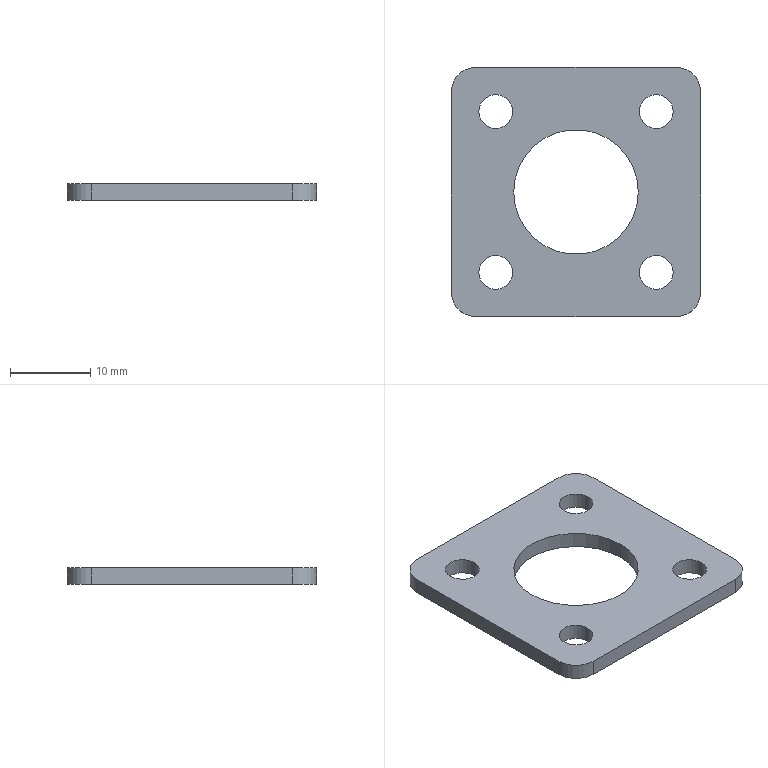Part | NX | features BREP 1 | 1 solid | 20 faces | box 31 x 31 x 2 mm | volume 1418 mm3 | cylinder 14 | plane 6 | commonest cylinder face diameters 4.2 x8 6 x4 15.5 x2
STEP:
#1=CARTESIAN_POINT('',(-258.211,-178.403,2108.));
#2=VERTEX_POINT('',#1);
#3=CARTESIAN_POINT('',(-262.411,-178.403,2108.));
#4=VERTEX_POINT('',#3);
#5=CARTESIAN_POINT('',(-260.311,-178.403,2108.));
#6=DIRECTION('',(0.,0.,-1.));
#7=DIRECTION('',(-1.,0.,0.));
#8=AXIS2_PLACEMENT_3D('',#5,#6,#7);
#9=CIRCLE('',#8,2.1);
#10=EDGE_CURVE('',#2,#4,#9,.T.);
#11=ORIENTED_EDGE('',*,*,#10,.F.);
#12=CARTESIAN_POINT('',(-258.211,-178.403,2106.));
#13=VERTEX_POINT('',#12);
#14=CARTESIAN_POINT('',(-258.211,-178.403,2108.));
#15=DIRECTION('',(0.,0.,-1.));
#16=VECTOR('',#15,1000.);
#17=LINE('',#14,#16);
#18=EDGE_CURVE('',#13,#2,#17,.F.);
#19=ORIENTED_EDGE('',*,*,#18,.F.);
#20=CARTESIAN_POINT('',(-262.411,-178.403,2106.));
#21=VERTEX_POINT('',#20);
#22=CARTESIAN_POINT('',(-260.311,-178.403,2106.));
#23=DIRECTION('',(0.,0.,1.));
#24=DIRECTION('',(-1.,0.,0.));
#25=AXIS2_PLACEMENT_3D('',#22,#23,#24);
#26=CIRCLE('',#25,2.1);
#27=EDGE_CURVE('',#21,#13,#26,.T.);
#28=ORIENTED_EDGE('',*,*,#27,.F.);
#29=CARTESIAN_POINT('',(-262.411,-178.403,2108.));
#30=DIRECTION('',(0.,0.,-1.));
#31=VECTOR('',#30,1000.);
#32=LINE('',#29,#31);
#33=EDGE_CURVE('',#21,#4,#32,.F.);
#34=ORIENTED_EDGE('',*,*,#33,.T.);
#35=EDGE_LOOP('',(#11,#19,#28,#34));
#36=FACE_BOUND('',#35,.T.);
#37=CARTESIAN_POINT('',(-260.311,-178.403,2108.));
#38=DIRECTION('',(0.,0.,-1.));
#39=DIRECTION('',(1.,0.,0.));
#40=AXIS2_PLACEMENT_3D('',#37,#38,#39);
#41=CYLINDRICAL_SURFACE('',#40,2.1);
#42=ADVANCED_FACE('',(#36),#41,.F.);
#43=CARTESIAN_POINT('',(-238.211,-198.403,2108.));
#44=VERTEX_POINT('',#43);
#45=CARTESIAN_POINT('',(-242.411,-198.403,2108.));
#46=VERTEX_POINT('',#45);
#47=CARTESIAN_POINT('',(-240.311,-198.403,2108.));
#48=DIRECTION('',(0.,0.,-1.));
#49=DIRECTION('',(-1.,0.,0.));
#50=AXIS2_PLACEMENT_3D('',#47,#48,#49);
#51=CIRCLE('',#50,2.1);
#52=EDGE_CURVE('',#44,#46,#51,.T.);
#53=ORIENTED_EDGE('',*,*,#52,.F.);
#54=CARTESIAN_POINT('',(-238.211,-198.403,2106.));
#55=VERTEX_POINT('',#54);
#56=CARTESIAN_POINT('',(-238.211,-198.403,2108.));
#57=DIRECTION('',(0.,0.,-1.));
#58=VECTOR('',#57,1000.);
#59=LINE('',#56,#58);
#60=EDGE_CURVE('',#55,#44,#59,.F.);
#61=ORIENTED_EDGE('',*,*,#60,.F.);
#62=CARTESIAN_POINT('',(-242.411,-198.403,2106.));
#63=VERTEX_POINT('',#62);
#64=CARTESIAN_POINT('',(-240.311,-198.403,2106.));
#65=DIRECTION('',(0.,0.,1.));
#66=DIRECTION('',(-1.,0.,0.));
#67=AXIS2_PLACEMENT_3D('',#64,#65,#66);
#68=CIRCLE('',#67,2.1);
#69=EDGE_CURVE('',#63,#55,#68,.T.);
#70=ORIENTED_EDGE('',*,*,#69,.F.);
#71=CARTESIAN_POINT('',(-242.411,-198.403,2108.));
#72=DIRECTION('',(0.,0.,-1.));
#73=VECTOR('',#72,1000.);
#74=LINE('',#71,#73);
#75=EDGE_CURVE('',#63,#46,#74,.F.);
#76=ORIENTED_EDGE('',*,*,#75,.T.);
#77=EDGE_LOOP('',(#53,#61,#70,#76));
#78=FACE_BOUND('',#77,.T.);
#79=CARTESIAN_POINT('',(-240.311,-198.403,2108.));
#80=DIRECTION('',(0.,0.,-1.));
#81=DIRECTION('',(1.,0.,0.));
#82=AXIS2_PLACEMENT_3D('',#79,#80,#81);
#83=CYLINDRICAL_SURFACE('',#82,2.1);
#84=ADVANCED_FACE('',(#78),#83,.F.);
#85=CARTESIAN_POINT('',(-242.561,-188.403,2108.));
#86=VERTEX_POINT('',#85);
#87=CARTESIAN_POINT('',(-258.061,-188.403,2108.));
#88=VERTEX_POINT('',#87);
#89=CARTESIAN_POINT('',(-250.311,-188.403,2108.));
#90=DIRECTION('',(0.,0.,-1.));
#91=DIRECTION('',(-1.,0.,0.));
#92=AXIS2_PLACEMENT_3D('',#89,#90,#91);
#93=CIRCLE('',#92,7.75);
#94=EDGE_CURVE('',#86,#88,#93,.T.);
#95=ORIENTED_EDGE('',*,*,#94,.F.);
#96=CARTESIAN_POINT('',(-242.561,-188.403,2106.));
#97=VERTEX_POINT('',#96);
#98=CARTESIAN_POINT('',(-242.561,-188.403,2108.));
#99=DIRECTION('',(0.,0.,-1.));
#100=VECTOR('',#99,1000.);
#101=LINE('',#98,#100);
#102=EDGE_CURVE('',#97,#86,#101,.F.);
#103=ORIENTED_EDGE('',*,*,#102,.F.);
#104=CARTESIAN_POINT('',(-258.061,-188.403,2106.));
#105=VERTEX_POINT('',#104);
#106=CARTESIAN_POINT('',(-250.311,-188.403,2106.));
#107=DIRECTION('',(0.,0.,1.));
#108=DIRECTION('',(-1.,0.,0.));
#109=AXIS2_PLACEMENT_3D('',#106,#107,#108);
#110=CIRCLE('',#109,7.75);
#111=EDGE_CURVE('',#105,#97,#110,.T.);
#112=ORIENTED_EDGE('',*,*,#111,.F.);
#113=CARTESIAN_POINT('',(-258.061,-188.403,2108.));
#114=DIRECTION('',(0.,0.,-1.));
#115=VECTOR('',#114,1000.);
#116=LINE('',#113,#115);
#117=EDGE_CURVE('',#105,#88,#116,.F.);
#118=ORIENTED_EDGE('',*,*,#117,.T.);
#119=EDGE_LOOP('',(#95,#103,#112,#118));
#120=FACE_BOUND('',#119,.T.);
#121=CARTESIAN_POINT('',(-250.311,-188.403,2108.));
#122=DIRECTION('',(0.,0.,-1.));
#123=DIRECTION('',(1.,0.,0.));
#124=AXIS2_PLACEMENT_3D('',#121,#122,#123);
#125=CYLINDRICAL_SURFACE('',#124,7.75);
#126=ADVANCED_FACE('',(#120),#125,.F.);
#127=CARTESIAN_POINT('',(-238.211,-178.403,2108.));
#128=VERTEX_POINT('',#127);
#129=CARTESIAN_POINT('',(-242.411,-178.403,2108.));
#130=VERTEX_POINT('',#129);
#131=CARTESIAN_POINT('',(-240.311,-178.403,2108.));
#132=DIRECTION('',(0.,0.,-1.));
#133=DIRECTION('',(-1.,0.,0.));
#134=AXIS2_PLACEMENT_3D('',#131,#132,#133);
#135=CIRCLE('',#134,2.1);
#136=EDGE_CURVE('',#128,#130,#135,.T.);
#137=ORIENTED_EDGE('',*,*,#136,.F.);
#138=CARTESIAN_POINT('',(-238.211,-178.403,2106.));
#139=VERTEX_POINT('',#138);
#140=CARTESIAN_POINT('',(-238.211,-178.403,2108.));
#141=DIRECTION('',(0.,0.,-1.));
#142=VECTOR('',#141,1000.);
#143=LINE('',#140,#142);
#144=EDGE_CURVE('',#139,#128,#143,.F.);
#145=ORIENTED_EDGE('',*,*,#144,.F.);
#146=CARTESIAN_POINT('',(-242.411,-178.403,2106.));
#147=VERTEX_POINT('',#146);
#148=CARTESIAN_POINT('',(-240.311,-178.403,2106.));
#149=DIRECTION('',(0.,0.,1.));
#150=DIRECTION('',(-1.,0.,0.));
#151=AXIS2_PLACEMENT_3D('',#148,#149,#150);
#152=CIRCLE('',#151,2.1);
#153=EDGE_CURVE('',#147,#139,#152,.T.);
#154=ORIENTED_EDGE('',*,*,#153,.F.);
#155=CARTESIAN_POINT('',(-242.411,-178.403,2108.));
#156=DIRECTION('',(0.,0.,-1.));
#157=VECTOR('',#156,1000.);
#158=LINE('',#155,#157);
#159=EDGE_CURVE('',#147,#130,#158,.F.);
#160=ORIENTED_EDGE('',*,*,#159,.T.);
#161=EDGE_LOOP('',(#137,#145,#154,#160));
#162=FACE_BOUND('',#161,.T.);
#163=CARTESIAN_POINT('',(-240.311,-178.403,2108.));
#164=DIRECTION('',(0.,0.,-1.));
#165=DIRECTION('',(1.,0.,0.));
#166=AXIS2_PLACEMENT_3D('',#163,#164,#165);
#167=CYLINDRICAL_SURFACE('',#166,2.1);
#168=ADVANCED_FACE('',(#162),#167,.F.);
#169=CARTESIAN_POINT('',(-258.211,-198.403,2108.));
#170=VERTEX_POINT('',#169);
#171=CARTESIAN_POINT('',(-262.411,-198.403,2108.));
#172=VERTEX_POINT('',#171);
#173=CARTESIAN_POINT('',(-260.311,-198.403,2108.));
#174=DIRECTION('',(0.,0.,-1.));
#175=DIRECTION('',(-1.,0.,0.));
#176=AXIS2_PLACEMENT_3D('',#173,#174,#175);
#177=CIRCLE('',#176,2.1);
#178=EDGE_CURVE('',#170,#172,#177,.T.);
#179=ORIENTED_EDGE('',*,*,#178,.F.);
#180=CARTESIAN_POINT('',(-258.211,-198.403,2106.));
#181=VERTEX_POINT('',#180);
#182=CARTESIAN_POINT('',(-258.211,-198.403,2108.));
#183=DIRECTION('',(0.,0.,-1.));
#184=VECTOR('',#183,1000.);
#185=LINE('',#182,#184);
#186=EDGE_CURVE('',#181,#170,#185,.F.);
#187=ORIENTED_EDGE('',*,*,#186,.F.);
#188=CARTESIAN_POINT('',(-262.411,-198.403,2106.));
#189=VERTEX_POINT('',#188);
#190=CARTESIAN_POINT('',(-260.311,-198.403,2106.));
#191=DIRECTION('',(0.,0.,1.));
#192=DIRECTION('',(-1.,0.,0.));
#193=AXIS2_PLACEMENT_3D('',#190,#191,#192);
#194=CIRCLE('',#193,2.1);
#195=EDGE_CURVE('',#189,#181,#194,.T.);
#196=ORIENTED_EDGE('',*,*,#195,.F.);
#197=CARTESIAN_POINT('',(-262.411,-198.403,2108.));
#198=DIRECTION('',(0.,0.,-1.));
#199=VECTOR('',#198,1000.);
#200=LINE('',#197,#199);
#201=EDGE_CURVE('',#189,#172,#200,.F.);
#202=ORIENTED_EDGE('',*,*,#201,.T.);
#203=EDGE_LOOP('',(#179,#187,#196,#202));
#204=FACE_BOUND('',#203,.T.);
#205=CARTESIAN_POINT('',(-260.311,-198.403,2108.));
#206=DIRECTION('',(0.,0.,-1.));
#207=DIRECTION('',(1.,0.,0.));
#208=AXIS2_PLACEMENT_3D('',#205,#206,#207);
#209=CYLINDRICAL_SURFACE('',#208,2.1);
#210=ADVANCED_FACE('',(#204),#209,.F.);
#211=CARTESIAN_POINT('',(-234.811,-175.903,2108.));
#212=VERTEX_POINT('',#211);
#213=CARTESIAN_POINT('',(-237.811,-172.903,2108.));
#214=VERTEX_POINT('',#213);
#215=CARTESIAN_POINT('',(-237.811,-175.903,2108.));
#216=DIRECTION('',(0.,0.,1.));
#217=DIRECTION('',(1.,0.,0.));
#218=AXIS2_PLACEMENT_3D('',#215,#216,#217);
#219=CIRCLE('',#218,3.);
#220=EDGE_CURVE('',#212,#214,#219,.T.);
#221=ORIENTED_EDGE('',*,*,#220,.T.);
#222=CARTESIAN_POINT('',(-262.811,-172.903,2108.));
#223=VERTEX_POINT('',#222);
#224=CARTESIAN_POINT('',(-237.311,-172.903,2108.));
#225=DIRECTION('',(-1.,0.,0.));
#226=VECTOR('',#225,1000.);
#227=LINE('',#224,#226);
#228=EDGE_CURVE('',#214,#223,#227,.T.);
#229=ORIENTED_EDGE('',*,*,#228,.T.);
#230=CARTESIAN_POINT('',(-265.811,-175.903,2108.));
#231=VERTEX_POINT('',#230);
#232=CARTESIAN_POINT('',(-262.811,-175.903,2108.));
#233=DIRECTION('',(0.,0.,1.));
#234=DIRECTION('',(1.,0.,0.));
#235=AXIS2_PLACEMENT_3D('',#232,#233,#234);
#236=CIRCLE('',#235,3.);
#237=EDGE_CURVE('',#223,#231,#236,.T.);
#238=ORIENTED_EDGE('',*,*,#237,.T.);
#239=CARTESIAN_POINT('',(-265.811,-200.903,2108.));
#240=VERTEX_POINT('',#239);
#241=CARTESIAN_POINT('',(-265.811,-201.403,2108.));
#242=DIRECTION('',(0.,-1.,0.));
#243=VECTOR('',#242,1000.);
#244=LINE('',#241,#243);
#245=EDGE_CURVE('',#231,#240,#244,.T.);
#246=ORIENTED_EDGE('',*,*,#245,.T.);
#247=CARTESIAN_POINT('',(-262.811,-203.903,2108.));
#248=VERTEX_POINT('',#247);
#249=CARTESIAN_POINT('',(-262.811,-200.903,2108.));
#250=DIRECTION('',(0.,0.,1.));
#251=DIRECTION('',(1.,0.,0.));
#252=AXIS2_PLACEMENT_3D('',#249,#250,#251);
#253=CIRCLE('',#252,3.);
#254=EDGE_CURVE('',#240,#248,#253,.T.);
#255=ORIENTED_EDGE('',*,*,#254,.T.);
#256=CARTESIAN_POINT('',(-237.811,-203.903,2108.));
#257=VERTEX_POINT('',#256);
#258=CARTESIAN_POINT('',(-237.311,-203.903,2108.));
#259=DIRECTION('',(1.,0.,0.));
#260=VECTOR('',#259,1000.);
#261=LINE('',#258,#260);
#262=EDGE_CURVE('',#248,#257,#261,.T.);
#263=ORIENTED_EDGE('',*,*,#262,.T.);
#264=CARTESIAN_POINT('',(-234.811,-200.903,2108.));
#265=VERTEX_POINT('',#264);
#266=CARTESIAN_POINT('',(-237.811,-200.903,2108.));
#267=DIRECTION('',(0.,0.,1.));
#268=DIRECTION('',(1.,0.,0.));
#269=AXIS2_PLACEMENT_3D('',#266,#267,#268);
#270=CIRCLE('',#269,3.);
#271=EDGE_CURVE('',#257,#265,#270,.T.);
#272=ORIENTED_EDGE('',*,*,#271,.T.);
#273=CARTESIAN_POINT('',(-234.811,-201.403,2108.));
#274=DIRECTION('',(0.,1.,0.));
#275=VECTOR('',#274,1000.);
#276=LINE('',#273,#275);
#277=EDGE_CURVE('',#265,#212,#276,.T.);
#278=ORIENTED_EDGE('',*,*,#277,.T.);
#279=EDGE_LOOP('',(#221,#229,#238,#246,#255,#263,#272,#278));
#280=FACE_BOUND('',#279,.T.);
#281=CARTESIAN_POINT('',(-260.311,-178.403,2108.));
#282=DIRECTION('',(0.,0.,-1.));
#283=DIRECTION('',(-1.,0.,0.));
#284=AXIS2_PLACEMENT_3D('',#281,#282,#283);
#285=CIRCLE('',#284,2.1);
#286=EDGE_CURVE('',#4,#2,#285,.T.);
#287=ORIENTED_EDGE('',*,*,#286,.T.);
#288=ORIENTED_EDGE('',*,*,#10,.T.);
#289=EDGE_LOOP('',(#287,#288));
#290=FACE_BOUND('',#289,.T.);
#291=CARTESIAN_POINT('',(-240.311,-198.403,2108.));
#292=DIRECTION('',(0.,0.,-1.));
#293=DIRECTION('',(-1.,0.,0.));
#294=AXIS2_PLACEMENT_3D('',#291,#292,#293);
#295=CIRCLE('',#294,2.1);
#296=EDGE_CURVE('',#46,#44,#295,.T.);
#297=ORIENTED_EDGE('',*,*,#296,.T.);
#298=ORIENTED_EDGE('',*,*,#52,.T.);
#299=EDGE_LOOP('',(#297,#298));
#300=FACE_BOUND('',#299,.T.);
#301=CARTESIAN_POINT('',(-250.311,-188.403,2108.));
#302=DIRECTION('',(0.,0.,-1.));
#303=DIRECTION('',(-1.,0.,0.));
#304=AXIS2_PLACEMENT_3D('',#301,#302,#303);
#305=CIRCLE('',#304,7.75);
#306=EDGE_CURVE('',#88,#86,#305,.T.);
#307=ORIENTED_EDGE('',*,*,#306,.T.);
#308=ORIENTED_EDGE('',*,*,#94,.T.);
#309=EDGE_LOOP('',(#307,#308));
#310=FACE_BOUND('',#309,.T.);
#311=CARTESIAN_POINT('',(-240.311,-178.403,2108.));
#312=DIRECTION('',(0.,0.,-1.));
#313=DIRECTION('',(-1.,0.,0.));
#314=AXIS2_PLACEMENT_3D('',#311,#312,#313);
#315=CIRCLE('',#314,2.1);
#316=EDGE_CURVE('',#130,#128,#315,.T.);
#317=ORIENTED_EDGE('',*,*,#316,.T.);
#318=ORIENTED_EDGE('',*,*,#136,.T.);
#319=EDGE_LOOP('',(#317,#318));
#320=FACE_BOUND('',#319,.T.);
#321=CARTESIAN_POINT('',(-260.311,-198.403,2108.));
#322=DIRECTION('',(0.,0.,-1.));
#323=DIRECTION('',(-1.,0.,0.));
#324=AXIS2_PLACEMENT_3D('',#321,#322,#323);
#325=CIRCLE('',#324,2.1);
#326=EDGE_CURVE('',#172,#170,#325,.T.);
#327=ORIENTED_EDGE('',*,*,#326,.T.);
#328=ORIENTED_EDGE('',*,*,#178,.T.);
#329=EDGE_LOOP('',(#327,#328));
#330=FACE_BOUND('',#329,.T.);
#331=CARTESIAN_POINT('',(-237.311,-201.403,2108.));
#332=DIRECTION('',(0.,0.,1.));
#333=DIRECTION('',(-1.,0.,0.));
#334=AXIS2_PLACEMENT_3D('',#331,#332,#333);
#335=PLANE('',#334);
#336=ADVANCED_FACE('',(#280,#290,#300,#310,#320,#330),#335,.T.);
#337=CARTESIAN_POINT('',(-237.811,-172.903,2106.));
#338=VERTEX_POINT('',#337);
#339=CARTESIAN_POINT('',(-237.811,-172.903,2098.));
#340=DIRECTION('',(0.,0.,1.));
#341=VECTOR('',#340,1000.);
#342=LINE('',#339,#341);
#343=EDGE_CURVE('',#338,#214,#342,.T.);
#344=ORIENTED_EDGE('',*,*,#343,.F.);
#345=CARTESIAN_POINT('',(-262.811,-172.903,2106.));
#346=VERTEX_POINT('',#345);
#347=CARTESIAN_POINT('',(-250.311,-172.903,2106.));
#348=DIRECTION('',(1.,0.,0.));
#349=VECTOR('',#348,1000.);
#350=LINE('',#347,#349);
#351=EDGE_CURVE('',#346,#338,#350,.T.);
#352=ORIENTED_EDGE('',*,*,#351,.F.);
#353=CARTESIAN_POINT('',(-262.811,-172.903,2098.));
#354=DIRECTION('',(0.,0.,-1.));
#355=VECTOR('',#354,1000.);
#356=LINE('',#353,#355);
#357=EDGE_CURVE('',#223,#346,#356,.T.);
#358=ORIENTED_EDGE('',*,*,#357,.F.);
#359=ORIENTED_EDGE('',*,*,#228,.F.);
#360=EDGE_LOOP('',(#344,#352,#358,#359));
#361=FACE_BOUND('',#360,.T.);
#362=CARTESIAN_POINT('',(-250.311,-172.903,2098.));
#363=DIRECTION('',(0.,-1.,0.));
#364=DIRECTION('',(0.,0.,1.));
#365=AXIS2_PLACEMENT_3D('',#362,#363,#364);
#366=PLANE('',#365);
#367=ADVANCED_FACE('',(#361),#366,.F.);
#368=ORIENTED_EDGE('',*,*,#343,.T.);
#369=ORIENTED_EDGE('',*,*,#220,.F.);
#370=CARTESIAN_POINT('',(-234.811,-175.903,2106.));
#371=VERTEX_POINT('',#370);
#372=CARTESIAN_POINT('',(-234.811,-175.903,2098.));
#373=DIRECTION('',(0.,0.,-1.));
#374=VECTOR('',#373,1000.);
#375=LINE('',#372,#374);
#376=EDGE_CURVE('',#212,#371,#375,.T.);
#377=ORIENTED_EDGE('',*,*,#376,.T.);
#378=CARTESIAN_POINT('',(-237.811,-175.903,2106.));
#379=DIRECTION('',(0.,0.,1.));
#380=DIRECTION('',(1.,0.,0.));
#381=AXIS2_PLACEMENT_3D('',#378,#379,#380);
#382=CIRCLE('',#381,3.);
#383=EDGE_CURVE('',#371,#338,#382,.T.);
#384=ORIENTED_EDGE('',*,*,#383,.T.);
#385=EDGE_LOOP('',(#368,#369,#377,#384));
#386=FACE_BOUND('',#385,.T.);
#387=CARTESIAN_POINT('',(-237.811,-175.903,2098.));
#388=DIRECTION('',(0.,0.,1.));
#389=DIRECTION('',(-1.,0.,0.));
#390=AXIS2_PLACEMENT_3D('',#387,#388,#389);
#391=CYLINDRICAL_SURFACE('',#390,3.);
#392=ADVANCED_FACE('',(#386),#391,.T.);
#393=ORIENTED_EDGE('',*,*,#277,.F.);
#394=CARTESIAN_POINT('',(-234.811,-200.903,2106.));
#395=VERTEX_POINT('',#394);
#396=CARTESIAN_POINT('',(-234.811,-200.903,2098.));
#397=DIRECTION('',(0.,0.,-1.));
#398=VECTOR('',#397,1000.);
#399=LINE('',#396,#398);
#400=EDGE_CURVE('',#265,#395,#399,.T.);
#401=ORIENTED_EDGE('',*,*,#400,.T.);
#402=CARTESIAN_POINT('',(-234.811,-188.403,2106.));
#403=DIRECTION('',(0.,1.,0.));
#404=VECTOR('',#403,1000.);
#405=LINE('',#402,#404);
#406=EDGE_CURVE('',#395,#371,#405,.T.);
#407=ORIENTED_EDGE('',*,*,#406,.T.);
#408=ORIENTED_EDGE('',*,*,#376,.F.);
#409=EDGE_LOOP('',(#393,#401,#407,#408));
#410=FACE_BOUND('',#409,.T.);
#411=CARTESIAN_POINT('',(-234.811,-188.403,2098.));
#412=DIRECTION('',(1.,0.,0.));
#413=DIRECTION('',(0.,0.,1.));
#414=AXIS2_PLACEMENT_3D('',#411,#412,#413);
#415=PLANE('',#414);
#416=ADVANCED_FACE('',(#410),#415,.T.);
#417=ORIENTED_EDGE('',*,*,#400,.F.);
#418=ORIENTED_EDGE('',*,*,#271,.F.);
#419=CARTESIAN_POINT('',(-237.811,-203.903,2106.));
#420=VERTEX_POINT('',#419);
#421=CARTESIAN_POINT('',(-237.811,-203.903,2098.));
#422=DIRECTION('',(0.,0.,-1.));
#423=VECTOR('',#422,1000.);
#424=LINE('',#421,#423);
#425=EDGE_CURVE('',#257,#420,#424,.T.);
#426=ORIENTED_EDGE('',*,*,#425,.T.);
#427=CARTESIAN_POINT('',(-237.811,-200.903,2106.));
#428=DIRECTION('',(0.,0.,1.));
#429=DIRECTION('',(1.,0.,0.));
#430=AXIS2_PLACEMENT_3D('',#427,#428,#429);
#431=CIRCLE('',#430,3.);
#432=EDGE_CURVE('',#420,#395,#431,.T.);
#433=ORIENTED_EDGE('',*,*,#432,.T.);
#434=EDGE_LOOP('',(#417,#418,#426,#433));
#435=FACE_BOUND('',#434,.T.);
#436=CARTESIAN_POINT('',(-237.811,-200.903,2098.));
#437=DIRECTION('',(0.,0.,1.));
#438=DIRECTION('',(-1.,0.,0.));
#439=AXIS2_PLACEMENT_3D('',#436,#437,#438);
#440=CYLINDRICAL_SURFACE('',#439,3.);
#441=ADVANCED_FACE('',(#435),#440,.T.);
#442=ORIENTED_EDGE('',*,*,#262,.F.);
#443=CARTESIAN_POINT('',(-262.811,-203.903,2106.));
#444=VERTEX_POINT('',#443);
#445=CARTESIAN_POINT('',(-262.811,-203.903,2098.));
#446=DIRECTION('',(0.,0.,-1.));
#447=VECTOR('',#446,1000.);
#448=LINE('',#445,#447);
#449=EDGE_CURVE('',#248,#444,#448,.T.);
#450=ORIENTED_EDGE('',*,*,#449,.T.);
#451=CARTESIAN_POINT('',(-250.311,-203.903,2106.));
#452=DIRECTION('',(1.,0.,0.));
#453=VECTOR('',#452,1000.);
#454=LINE('',#451,#453);
#455=EDGE_CURVE('',#444,#420,#454,.T.);
#456=ORIENTED_EDGE('',*,*,#455,.T.);
#457=ORIENTED_EDGE('',*,*,#425,.F.);
#458=EDGE_LOOP('',(#442,#450,#456,#457));
#459=FACE_BOUND('',#458,.T.);
#460=CARTESIAN_POINT('',(-250.311,-203.903,2098.));
#461=DIRECTION('',(0.,-1.,0.));
#462=DIRECTION('',(0.,0.,1.));
#463=AXIS2_PLACEMENT_3D('',#460,#461,#462);
#464=PLANE('',#463);
#465=ADVANCED_FACE('',(#459),#464,.T.);
#466=ORIENTED_EDGE('',*,*,#449,.F.);
#467=ORIENTED_EDGE('',*,*,#254,.F.);
#468=CARTESIAN_POINT('',(-265.811,-200.903,2106.));
#469=VERTEX_POINT('',#468);
#470=CARTESIAN_POINT('',(-265.811,-200.903,2098.));
#471=DIRECTION('',(0.,0.,-1.));
#472=VECTOR('',#471,1000.);
#473=LINE('',#470,#472);
#474=EDGE_CURVE('',#240,#469,#473,.T.);
#475=ORIENTED_EDGE('',*,*,#474,.T.);
#476=CARTESIAN_POINT('',(-262.811,-200.903,2106.));
#477=DIRECTION('',(0.,0.,1.));
#478=DIRECTION('',(1.,0.,0.));
#479=AXIS2_PLACEMENT_3D('',#476,#477,#478);
#480=CIRCLE('',#479,3.);
#481=EDGE_CURVE('',#469,#444,#480,.T.);
#482=ORIENTED_EDGE('',*,*,#481,.T.);
#483=EDGE_LOOP('',(#466,#467,#475,#482));
#484=FACE_BOUND('',#483,.T.);
#485=CARTESIAN_POINT('',(-262.811,-200.903,2098.));
#486=DIRECTION('',(0.,0.,1.));
#487=DIRECTION('',(-1.,0.,0.));
#488=AXIS2_PLACEMENT_3D('',#485,#486,#487);
#489=CYLINDRICAL_SURFACE('',#488,3.);
#490=ADVANCED_FACE('',(#484),#489,.T.);
#491=ORIENTED_EDGE('',*,*,#245,.F.);
#492=CARTESIAN_POINT('',(-265.811,-175.903,2106.));
#493=VERTEX_POINT('',#492);
#494=CARTESIAN_POINT('',(-265.811,-175.903,2098.));
#495=DIRECTION('',(0.,0.,1.));
#496=VECTOR('',#495,1000.);
#497=LINE('',#494,#496);
#498=EDGE_CURVE('',#493,#231,#497,.T.);
#499=ORIENTED_EDGE('',*,*,#498,.F.);
#500=CARTESIAN_POINT('',(-265.811,-188.403,2106.));
#501=DIRECTION('',(0.,1.,0.));
#502=VECTOR('',#501,1000.);
#503=LINE('',#500,#502);
#504=EDGE_CURVE('',#469,#493,#503,.T.);
#505=ORIENTED_EDGE('',*,*,#504,.F.);
#506=ORIENTED_EDGE('',*,*,#474,.F.);
#507=EDGE_LOOP('',(#491,#499,#505,#506));
#508=FACE_BOUND('',#507,.T.);
#509=CARTESIAN_POINT('',(-265.811,-188.403,2098.));
#510=DIRECTION('',(1.,0.,0.));
#511=DIRECTION('',(0.,0.,1.));
#512=AXIS2_PLACEMENT_3D('',#509,#510,#511);
#513=PLANE('',#512);
#514=ADVANCED_FACE('',(#508),#513,.F.);
#515=ORIENTED_EDGE('',*,*,#498,.T.);
#516=ORIENTED_EDGE('',*,*,#237,.F.);
#517=ORIENTED_EDGE('',*,*,#357,.T.);
#518=CARTESIAN_POINT('',(-262.811,-175.903,2106.));
#519=DIRECTION('',(0.,0.,1.));
#520=DIRECTION('',(1.,0.,0.));
#521=AXIS2_PLACEMENT_3D('',#518,#519,#520);
#522=CIRCLE('',#521,3.);
#523=EDGE_CURVE('',#346,#493,#522,.T.);
#524=ORIENTED_EDGE('',*,*,#523,.T.);
#525=EDGE_LOOP('',(#515,#516,#517,#524));
#526=FACE_BOUND('',#525,.T.);
#527=CARTESIAN_POINT('',(-262.811,-175.903,2098.));
#528=DIRECTION('',(0.,0.,1.));
#529=DIRECTION('',(-1.,0.,0.));
#530=AXIS2_PLACEMENT_3D('',#527,#528,#529);
#531=CYLINDRICAL_SURFACE('',#530,3.);
#532=ADVANCED_FACE('',(#526),#531,.T.);
#533=ORIENTED_EDGE('',*,*,#18,.T.);
#534=ORIENTED_EDGE('',*,*,#286,.F.);
#535=ORIENTED_EDGE('',*,*,#33,.F.);
#536=CARTESIAN_POINT('',(-260.311,-178.403,2106.));
#537=DIRECTION('',(0.,0.,1.));
#538=DIRECTION('',(-1.,0.,0.));
#539=AXIS2_PLACEMENT_3D('',#536,#537,#538);
#540=CIRCLE('',#539,2.1);
#541=EDGE_CURVE('',#13,#21,#540,.T.);
#542=ORIENTED_EDGE('',*,*,#541,.F.);
#543=EDGE_LOOP('',(#533,#534,#535,#542));
#544=FACE_BOUND('',#543,.T.);
#545=CARTESIAN_POINT('',(-260.311,-178.403,2108.));
#546=DIRECTION('',(0.,0.,-1.));
#547=DIRECTION('',(1.,0.,0.));
#548=AXIS2_PLACEMENT_3D('',#545,#546,#547);
#549=CYLINDRICAL_SURFACE('',#548,2.1);
#550=ADVANCED_FACE('',(#544),#549,.F.);
#551=ORIENTED_EDGE('',*,*,#60,.T.);
#552=ORIENTED_EDGE('',*,*,#296,.F.);
#553=ORIENTED_EDGE('',*,*,#75,.F.);
#554=CARTESIAN_POINT('',(-240.311,-198.403,2106.));
#555=DIRECTION('',(0.,0.,1.));
#556=DIRECTION('',(-1.,0.,0.));
#557=AXIS2_PLACEMENT_3D('',#554,#555,#556);
#558=CIRCLE('',#557,2.1);
#559=EDGE_CURVE('',#55,#63,#558,.T.);
#560=ORIENTED_EDGE('',*,*,#559,.F.);
#561=EDGE_LOOP('',(#551,#552,#553,#560));
#562=FACE_BOUND('',#561,.T.);
#563=CARTESIAN_POINT('',(-240.311,-198.403,2108.));
#564=DIRECTION('',(0.,0.,-1.));
#565=DIRECTION('',(1.,0.,0.));
#566=AXIS2_PLACEMENT_3D('',#563,#564,#565);
#567=CYLINDRICAL_SURFACE('',#566,2.1);
#568=ADVANCED_FACE('',(#562),#567,.F.);
#569=ORIENTED_EDGE('',*,*,#102,.T.);
#570=ORIENTED_EDGE('',*,*,#306,.F.);
#571=ORIENTED_EDGE('',*,*,#117,.F.);
#572=CARTESIAN_POINT('',(-250.311,-188.403,2106.));
#573=DIRECTION('',(0.,0.,1.));
#574=DIRECTION('',(-1.,0.,0.));
#575=AXIS2_PLACEMENT_3D('',#572,#573,#574);
#576=CIRCLE('',#575,7.75);
#577=EDGE_CURVE('',#97,#105,#576,.T.);
#578=ORIENTED_EDGE('',*,*,#577,.F.);
#579=EDGE_LOOP('',(#569,#570,#571,#578));
#580=FACE_BOUND('',#579,.T.);
#581=CARTESIAN_POINT('',(-250.311,-188.403,2108.));
#582=DIRECTION('',(0.,0.,-1.));
#583=DIRECTION('',(1.,0.,0.));
#584=AXIS2_PLACEMENT_3D('',#581,#582,#583);
#585=CYLINDRICAL_SURFACE('',#584,7.75);
#586=ADVANCED_FACE('',(#580),#585,.F.);
#587=ORIENTED_EDGE('',*,*,#144,.T.);
#588=ORIENTED_EDGE('',*,*,#316,.F.);
#589=ORIENTED_EDGE('',*,*,#159,.F.);
#590=CARTESIAN_POINT('',(-240.311,-178.403,2106.));
#591=DIRECTION('',(0.,0.,1.));
#592=DIRECTION('',(-1.,0.,0.));
#593=AXIS2_PLACEMENT_3D('',#590,#591,#592);
#594=CIRCLE('',#593,2.1);
#595=EDGE_CURVE('',#139,#147,#594,.T.);
#596=ORIENTED_EDGE('',*,*,#595,.F.);
#597=EDGE_LOOP('',(#587,#588,#589,#596));
#598=FACE_BOUND('',#597,.T.);
#599=CARTESIAN_POINT('',(-240.311,-178.403,2108.));
#600=DIRECTION('',(0.,0.,-1.));
#601=DIRECTION('',(1.,0.,0.));
#602=AXIS2_PLACEMENT_3D('',#599,#600,#601);
#603=CYLINDRICAL_SURFACE('',#602,2.1);
#604=ADVANCED_FACE('',(#598),#603,.F.);
#605=ORIENTED_EDGE('',*,*,#186,.T.);
#606=ORIENTED_EDGE('',*,*,#326,.F.);
#607=ORIENTED_EDGE('',*,*,#201,.F.);
#608=CARTESIAN_POINT('',(-260.311,-198.403,2106.));
#609=DIRECTION('',(0.,0.,1.));
#610=DIRECTION('',(-1.,0.,0.));
#611=AXIS2_PLACEMENT_3D('',#608,#609,#610);
#612=CIRCLE('',#611,2.1);
#613=EDGE_CURVE('',#181,#189,#612,.T.);
#614=ORIENTED_EDGE('',*,*,#613,.F.);
#615=EDGE_LOOP('',(#605,#606,#607,#614));
#616=FACE_BOUND('',#615,.T.);
#617=CARTESIAN_POINT('',(-260.311,-198.403,2108.));
#618=DIRECTION('',(0.,0.,-1.));
#619=DIRECTION('',(1.,0.,0.));
#620=AXIS2_PLACEMENT_3D('',#617,#618,#619);
#621=CYLINDRICAL_SURFACE('',#620,2.1);
#622=ADVANCED_FACE('',(#616),#621,.F.);
#623=ORIENTED_EDGE('',*,*,#383,.F.);
#624=ORIENTED_EDGE('',*,*,#406,.F.);
#625=ORIENTED_EDGE('',*,*,#432,.F.);
#626=ORIENTED_EDGE('',*,*,#455,.F.);
#627=ORIENTED_EDGE('',*,*,#481,.F.);
#628=ORIENTED_EDGE('',*,*,#504,.T.);
#629=ORIENTED_EDGE('',*,*,#523,.F.);
#630=ORIENTED_EDGE('',*,*,#351,.T.);
#631=EDGE_LOOP('',(#623,#624,#625,#626,#627,#628,#629,#630));
#632=FACE_BOUND('',#631,.T.);
#633=ORIENTED_EDGE('',*,*,#27,.T.);
#634=ORIENTED_EDGE('',*,*,#541,.T.);
#635=EDGE_LOOP('',(#633,#634));
#636=FACE_BOUND('',#635,.T.);
#637=ORIENTED_EDGE('',*,*,#195,.T.);
#638=ORIENTED_EDGE('',*,*,#613,.T.);
#639=EDGE_LOOP('',(#637,#638));
#640=FACE_BOUND('',#639,.T.);
#641=ORIENTED_EDGE('',*,*,#69,.T.);
#642=ORIENTED_EDGE('',*,*,#559,.T.);
#643=EDGE_LOOP('',(#641,#642));
#644=FACE_BOUND('',#643,.T.);
#645=ORIENTED_EDGE('',*,*,#153,.T.);
#646=ORIENTED_EDGE('',*,*,#595,.T.);
#647=EDGE_LOOP('',(#645,#646));
#648=FACE_BOUND('',#647,.T.);
#649=ORIENTED_EDGE('',*,*,#111,.T.);
#650=ORIENTED_EDGE('',*,*,#577,.T.);
#651=EDGE_LOOP('',(#649,#650));
#652=FACE_BOUND('',#651,.T.);
#653=CARTESIAN_POINT('',(-237.311,-201.403,2106.));
#654=DIRECTION('',(0.,0.,1.));
#655=DIRECTION('',(-1.,0.,0.));
#656=AXIS2_PLACEMENT_3D('',#653,#654,#655);
#657=PLANE('',#656);
#658=ADVANCED_FACE('',(#632,#636,#640,#644,#648,#652),#657,.F.);
#659=CLOSED_SHELL('',(#42,#84,#126,#168,#210,#336,#367,#392,#416,#441,#465,#490,#514,#532,#550,#568,#586,#604,#622,#658));
#660=MANIFOLD_SOLID_BREP('',#659);
#661=(LENGTH_UNIT()NAMED_UNIT(*)SI_UNIT(.MILLI.,.METRE.));
#662=UNCERTAINTY_MEASURE_WITH_UNIT(LENGTH_MEASURE(0.00001),#661,'','');
#663=(NAMED_UNIT(*)PLANE_ANGLE_UNIT()SI_UNIT($,.RADIAN.));
#664=(NAMED_UNIT(*)SI_UNIT($,.STERADIAN.)SOLID_ANGLE_UNIT());
#665=(GEOMETRIC_REPRESENTATION_CONTEXT(3)GLOBAL_UNCERTAINTY_ASSIGNED_CONTEXT((#662))GLOBAL_UNIT_ASSIGNED_CONTEXT((#661,#663,#664))REPRESENTATION_CONTEXT('',''));
#666=ADVANCED_BREP_SHAPE_REPRESENTATION('',(#660),#665);